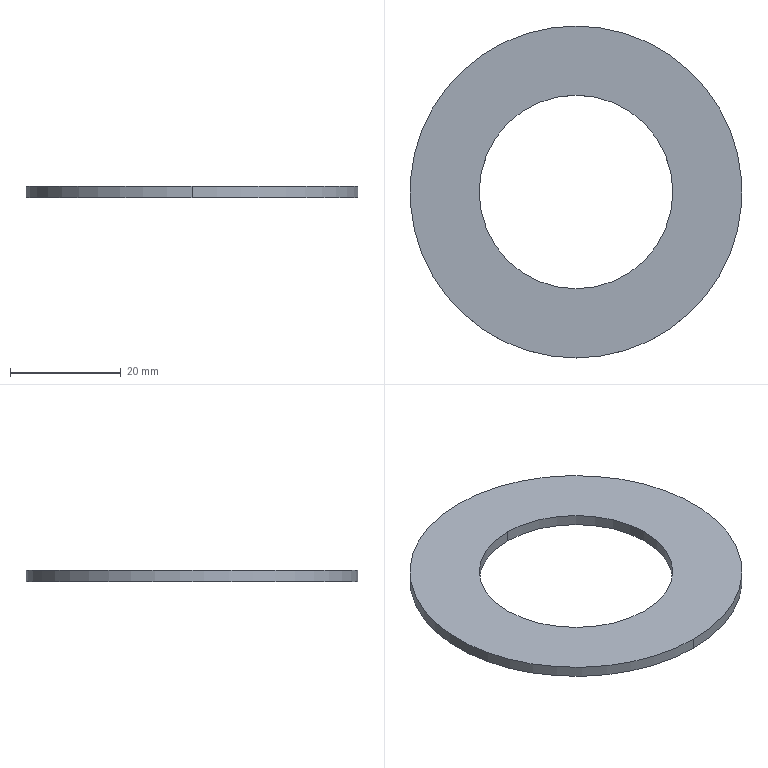Part | SolidWorks | features BaseBody 1 | 1 solid | 6 faces | box 60 x 60 x 2 mm | volume 3731 mm3 | cylinder 4 | plane 2 | commonest cylinder face diameters 35 x2 60 x2
STEP:
#1=CARTESIAN_POINT('',(591.519,-217.648,38.789));
#2=VERTEX_POINT('',#1);
#3=CARTESIAN_POINT('',(591.519,-157.648,38.789));
#4=VERTEX_POINT('',#3);
#5=CARTESIAN_POINT('',(591.519,-187.648,38.789));
#6=DIRECTION('',(0.,0.,1.));
#7=DIRECTION('',(0.,1.,0.));
#8=AXIS2_PLACEMENT_3D('',#5,#6,#7);
#9=CIRCLE('',#8,30.);
#10=EDGE_CURVE('',#2,#4,#9,.T.);
#11=ORIENTED_EDGE('',*,*,#10,.F.);
#12=CARTESIAN_POINT('',(591.519,-217.648,36.789));
#13=VERTEX_POINT('',#12);
#14=CARTESIAN_POINT('',(591.519,-217.648,36.789));
#15=DIRECTION('',(0.,0.,-1.));
#16=VECTOR('',#15,1000.);
#17=LINE('',#14,#16);
#18=EDGE_CURVE('',#2,#13,#17,.T.);
#19=ORIENTED_EDGE('',*,*,#18,.T.);
#20=CARTESIAN_POINT('',(591.519,-157.648,36.789));
#21=VERTEX_POINT('',#20);
#22=CARTESIAN_POINT('',(591.519,-187.648,36.789));
#23=DIRECTION('',(0.,0.,1.));
#24=DIRECTION('',(0.,1.,0.));
#25=AXIS2_PLACEMENT_3D('',#22,#23,#24);
#26=CIRCLE('',#25,30.);
#27=EDGE_CURVE('',#13,#21,#26,.T.);
#28=ORIENTED_EDGE('',*,*,#27,.T.);
#29=CARTESIAN_POINT('',(591.519,-157.648,36.789));
#30=DIRECTION('',(0.,0.,-1.));
#31=VECTOR('',#30,1000.);
#32=LINE('',#29,#31);
#33=EDGE_CURVE('',#4,#21,#32,.T.);
#34=ORIENTED_EDGE('',*,*,#33,.F.);
#35=EDGE_LOOP('',(#11,#19,#28,#34));
#36=FACE_OUTER_BOUND('',#35,.T.);
#37=CARTESIAN_POINT('',(591.519,-187.648,36.789));
#38=DIRECTION('',(0.,0.,-1.));
#39=DIRECTION('',(0.,1.,0.));
#40=AXIS2_PLACEMENT_3D('',#37,#38,#39);
#41=CYLINDRICAL_SURFACE('',#40,30.);
#42=ADVANCED_FACE('',(#36),#41,.T.);
#43=CARTESIAN_POINT('',(591.519,-170.148,36.789));
#44=VERTEX_POINT('',#43);
#45=CARTESIAN_POINT('',(591.519,-205.148,36.789));
#46=VERTEX_POINT('',#45);
#47=CARTESIAN_POINT('',(591.519,-187.648,36.789));
#48=DIRECTION('',(0.,0.,1.));
#49=DIRECTION('',(0.,-1.,0.));
#50=AXIS2_PLACEMENT_3D('',#47,#48,#49);
#51=CIRCLE('',#50,17.5);
#52=EDGE_CURVE('',#44,#46,#51,.T.);
#53=ORIENTED_EDGE('',*,*,#52,.F.);
#54=CARTESIAN_POINT('',(591.519,-170.148,38.789));
#55=VERTEX_POINT('',#54);
#56=CARTESIAN_POINT('',(591.519,-170.148,38.789));
#57=DIRECTION('',(0.,0.,1.));
#58=VECTOR('',#57,1000.);
#59=LINE('',#56,#58);
#60=EDGE_CURVE('',#44,#55,#59,.T.);
#61=ORIENTED_EDGE('',*,*,#60,.T.);
#62=CARTESIAN_POINT('',(591.519,-205.148,38.789));
#63=VERTEX_POINT('',#62);
#64=CARTESIAN_POINT('',(591.519,-187.648,38.789));
#65=DIRECTION('',(0.,0.,-1.));
#66=DIRECTION('',(0.,-1.,0.));
#67=AXIS2_PLACEMENT_3D('',#64,#65,#66);
#68=CIRCLE('',#67,17.5);
#69=EDGE_CURVE('',#63,#55,#68,.T.);
#70=ORIENTED_EDGE('',*,*,#69,.F.);
#71=CARTESIAN_POINT('',(591.519,-205.148,38.789));
#72=DIRECTION('',(0.,0.,1.));
#73=VECTOR('',#72,1000.);
#74=LINE('',#71,#73);
#75=EDGE_CURVE('',#46,#63,#74,.T.);
#76=ORIENTED_EDGE('',*,*,#75,.F.);
#77=EDGE_LOOP('',(#53,#61,#70,#76));
#78=FACE_OUTER_BOUND('',#77,.T.);
#79=CARTESIAN_POINT('',(591.519,-187.648,38.789));
#80=DIRECTION('',(0.,0.,1.));
#81=DIRECTION('',(0.,-1.,0.));
#82=AXIS2_PLACEMENT_3D('',#79,#80,#81);
#83=CYLINDRICAL_SURFACE('',#82,17.5);
#84=ADVANCED_FACE('',(#78),#83,.F.);
#85=CARTESIAN_POINT('',(591.519,-187.648,38.789));
#86=DIRECTION('',(0.,0.,1.));
#87=DIRECTION('',(0.,1.,0.));
#88=AXIS2_PLACEMENT_3D('',#85,#86,#87);
#89=CIRCLE('',#88,30.);
#90=EDGE_CURVE('',#4,#2,#89,.T.);
#91=ORIENTED_EDGE('',*,*,#90,.T.);
#92=ORIENTED_EDGE('',*,*,#10,.T.);
#93=EDGE_LOOP('',(#91,#92));
#94=FACE_OUTER_BOUND('',#93,.T.);
#95=ORIENTED_EDGE('',*,*,#69,.T.);
#96=CARTESIAN_POINT('',(591.519,-187.648,38.789));
#97=DIRECTION('',(0.,0.,-1.));
#98=DIRECTION('',(0.,-1.,0.));
#99=AXIS2_PLACEMENT_3D('',#96,#97,#98);
#100=CIRCLE('',#99,17.5);
#101=EDGE_CURVE('',#55,#63,#100,.T.);
#102=ORIENTED_EDGE('',*,*,#101,.T.);
#103=EDGE_LOOP('',(#95,#102));
#104=FACE_BOUND('',#103,.T.);
#105=CARTESIAN_POINT('',(591.519,-187.648,38.789));
#106=DIRECTION('',(0.,0.,1.));
#107=DIRECTION('',(0.,-1.,0.));
#108=AXIS2_PLACEMENT_3D('',#105,#106,#107);
#109=PLANE('',#108);
#110=ADVANCED_FACE('',(#94,#104),#109,.T.);
#111=ORIENTED_EDGE('',*,*,#18,.F.);
#112=ORIENTED_EDGE('',*,*,#90,.F.);
#113=ORIENTED_EDGE('',*,*,#33,.T.);
#114=CARTESIAN_POINT('',(591.519,-187.648,36.789));
#115=DIRECTION('',(0.,0.,1.));
#116=DIRECTION('',(0.,1.,0.));
#117=AXIS2_PLACEMENT_3D('',#114,#115,#116);
#118=CIRCLE('',#117,30.);
#119=EDGE_CURVE('',#21,#13,#118,.T.);
#120=ORIENTED_EDGE('',*,*,#119,.T.);
#121=EDGE_LOOP('',(#111,#112,#113,#120));
#122=FACE_OUTER_BOUND('',#121,.T.);
#123=CARTESIAN_POINT('',(591.519,-187.648,36.789));
#124=DIRECTION('',(0.,0.,-1.));
#125=DIRECTION('',(0.,1.,0.));
#126=AXIS2_PLACEMENT_3D('',#123,#124,#125);
#127=CYLINDRICAL_SURFACE('',#126,30.);
#128=ADVANCED_FACE('',(#122),#127,.T.);
#129=ORIENTED_EDGE('',*,*,#60,.F.);
#130=CARTESIAN_POINT('',(591.519,-187.648,36.789));
#131=DIRECTION('',(0.,0.,1.));
#132=DIRECTION('',(0.,-1.,0.));
#133=AXIS2_PLACEMENT_3D('',#130,#131,#132);
#134=CIRCLE('',#133,17.5);
#135=EDGE_CURVE('',#46,#44,#134,.T.);
#136=ORIENTED_EDGE('',*,*,#135,.F.);
#137=ORIENTED_EDGE('',*,*,#75,.T.);
#138=ORIENTED_EDGE('',*,*,#101,.F.);
#139=EDGE_LOOP('',(#129,#136,#137,#138));
#140=FACE_OUTER_BOUND('',#139,.T.);
#141=CARTESIAN_POINT('',(591.519,-187.648,38.789));
#142=DIRECTION('',(0.,0.,1.));
#143=DIRECTION('',(0.,-1.,0.));
#144=AXIS2_PLACEMENT_3D('',#141,#142,#143);
#145=CYLINDRICAL_SURFACE('',#144,17.5);
#146=ADVANCED_FACE('',(#140),#145,.F.);
#147=ORIENTED_EDGE('',*,*,#119,.F.);
#148=ORIENTED_EDGE('',*,*,#27,.F.);
#149=EDGE_LOOP('',(#147,#148));
#150=FACE_OUTER_BOUND('',#149,.T.);
#151=ORIENTED_EDGE('',*,*,#135,.T.);
#152=ORIENTED_EDGE('',*,*,#52,.T.);
#153=EDGE_LOOP('',(#151,#152));
#154=FACE_BOUND('',#153,.T.);
#155=CARTESIAN_POINT('',(591.519,-187.648,36.789));
#156=DIRECTION('',(0.,0.,1.));
#157=DIRECTION('',(0.,-1.,0.));
#158=AXIS2_PLACEMENT_3D('',#155,#156,#157);
#159=PLANE('',#158);
#160=ADVANCED_FACE('',(#150,#154),#159,.F.);
#161=CLOSED_SHELL('',(#42,#84,#110,#128,#146,#160));
#162=MANIFOLD_SOLID_BREP('',#161);
#163=CARTESIAN_POINT('',(0.,0.,0.));
#164=DIRECTION('',(0.,0.,1.));
#165=DIRECTION('',(1.,0.,0.));
#166=AXIS2_PLACEMENT_3D('',#163,#164,#165);
#167=(LENGTH_UNIT()NAMED_UNIT(*)SI_UNIT(.MILLI.,.METRE.));
#168=UNCERTAINTY_MEASURE_WITH_UNIT(LENGTH_MEASURE(0.00001),#167,'','');
#169=(NAMED_UNIT(*)PLANE_ANGLE_UNIT()SI_UNIT($,.RADIAN.));
#170=(NAMED_UNIT(*)SI_UNIT($,.STERADIAN.)SOLID_ANGLE_UNIT());
#171=(GEOMETRIC_REPRESENTATION_CONTEXT(3)GLOBAL_UNCERTAINTY_ASSIGNED_CONTEXT((#168))GLOBAL_UNIT_ASSIGNED_CONTEXT((#167,#169,#170))REPRESENTATION_CONTEXT('',''));
#172=ADVANCED_BREP_SHAPE_REPRESENTATION('',(#162,#166),#171);